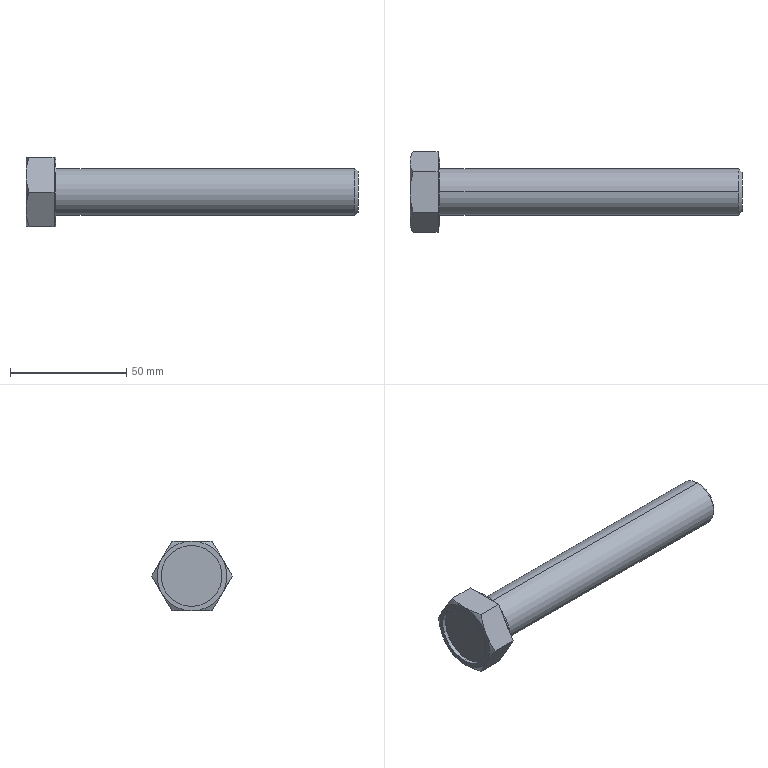Part | STEP file | formed hex screw_am_B18.2.3.2M - Formed hex screw, M20 x 2.5 x 130 --52WN | 1 solid | 30 faces | box 142.88 x 34.641 x 30 mm | volume 49864 mm3 | plane 16 | cone 8 | cylinder 6 | commonest cylinder face diameters 20 x2 26.25 x2 30 x2